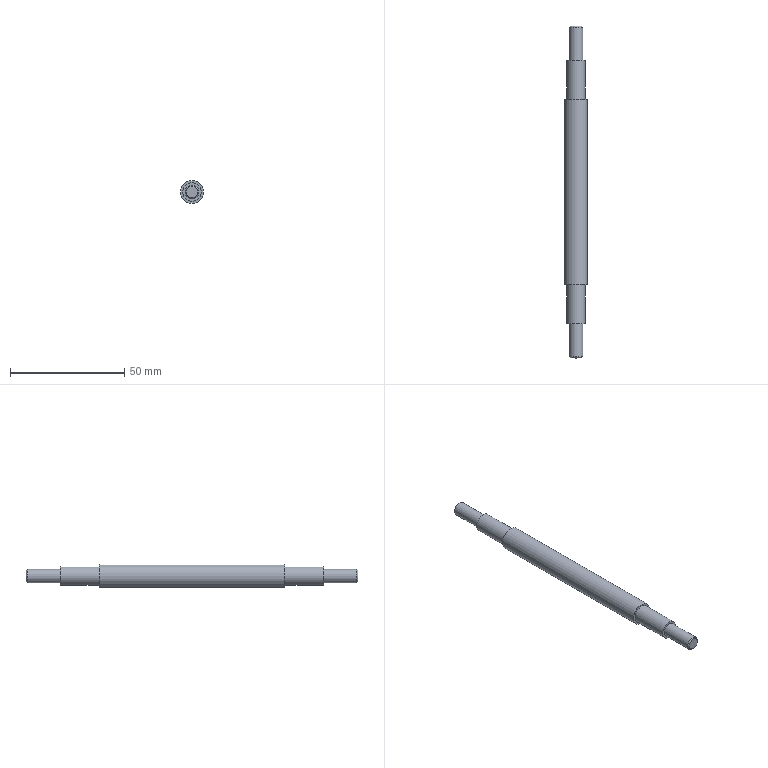Part | STEP file | 2-13.2 | 1 solid | 13 faces | box 10 x 145 x 10 mm | volume 8915 mm3 | plane 6 | cylinder 5 | cone 2 | commonest cylinder face diameters 6 x2 8 x2 10 x1
STEP:
#1=CARTESIAN_POINT('',(0.,0.,0.));
#2=DIRECTION('',(0.,0.,1.));
#3=DIRECTION('',(1.,0.,0.));
#4=AXIS2_PLACEMENT_3D('',#1,#2,#3);
#5=CARTESIAN_POINT('',(5.,40.5,0.));
#6=VERTEX_POINT('',#5);
#7=CARTESIAN_POINT('',(0.,40.5,0.));
#8=DIRECTION('',(0.,-1.,0.));
#9=DIRECTION('',(1.,0.,0.));
#10=AXIS2_PLACEMENT_3D('',#7,#8,#9);
#11=CIRCLE('',#10,5.);
#12=CARTESIAN_POINT('',(0.,40.5,0.));
#13=DIRECTION('',(0.,-1.,0.));
#14=DIRECTION('',(1.,0.,0.));
#15=AXIS2_PLACEMENT_3D('',#12,#13,#14);
#16=CYLINDRICAL_SURFACE('',#15,5.);
#17=CARTESIAN_POINT('',(0.,0.));
#18=DIRECTION('',(1.,0.));
#19=VECTOR('',#18,1.);
#20=LINE('',#17,#19);
#21=(GEOMETRIC_REPRESENTATION_CONTEXT(2)PARAMETRIC_REPRESENTATION_CONTEXT()REPRESENTATION_CONTEXT('',''));
#22=DEFINITIONAL_REPRESENTATION('',(#20),#21);
#23=PCURVE('',#16,#22);
#24=CARTESIAN_POINT('',(-1.34,40.5,0.));
#25=DIRECTION('',(0.,-1.,0.));
#26=DIRECTION('',(1.,0.,0.));
#27=AXIS2_PLACEMENT_3D('',#24,#25,#26);
#28=PLANE('',#27);
#29=CARTESIAN_POINT('',(1.34,0.));
#30=DIRECTION('',(1.,0.));
#31=AXIS2_PLACEMENT_2D('',#29,#30);
#32=CIRCLE('',#31,5.);
#33=(GEOMETRIC_REPRESENTATION_CONTEXT(2)PARAMETRIC_REPRESENTATION_CONTEXT()REPRESENTATION_CONTEXT('',''));
#34=DEFINITIONAL_REPRESENTATION('',(#32),#33);
#35=PCURVE('',#28,#34);
#36=SURFACE_CURVE('',#11,(#23,#35),.PCURVE_S1.);
#37=EDGE_CURVE('',#6,#6,#36,.T.);
#38=ORIENTED_EDGE('',*,*,#37,.T.);
#39=CARTESIAN_POINT('',(5.,-40.5,0.));
#40=VERTEX_POINT('',#39);
#41=CARTESIAN_POINT('',(5.,40.5,0.));
#42=DIRECTION('',(0.,-1.,0.));
#43=VECTOR('',#42,1.);
#44=LINE('',#41,#43);
#45=CARTESIAN_POINT('',(6.283,0.));
#46=DIRECTION('',(0.,1.));
#47=VECTOR('',#46,1.);
#48=LINE('',#45,#47);
#49=(GEOMETRIC_REPRESENTATION_CONTEXT(2)PARAMETRIC_REPRESENTATION_CONTEXT()REPRESENTATION_CONTEXT('',''));
#50=DEFINITIONAL_REPRESENTATION('',(#48),#49);
#51=PCURVE('',#16,#50);
#52=CARTESIAN_POINT('',(0.,0.));
#53=DIRECTION('',(0.,1.));
#54=VECTOR('',#53,1.);
#55=LINE('',#52,#54);
#56=(GEOMETRIC_REPRESENTATION_CONTEXT(2)PARAMETRIC_REPRESENTATION_CONTEXT()REPRESENTATION_CONTEXT('',''));
#57=DEFINITIONAL_REPRESENTATION('',(#55),#56);
#58=PCURVE('',#16,#57);
#59=SEAM_CURVE('',#44,(#51,#58),.PCURVE_S1.);
#60=EDGE_CURVE('',#6,#40,#59,.T.);
#61=ORIENTED_EDGE('',*,*,#60,.T.);
#62=CARTESIAN_POINT('',(0.,-40.5,0.));
#63=DIRECTION('',(0.,-1.,0.));
#64=DIRECTION('',(1.,0.,0.));
#65=AXIS2_PLACEMENT_3D('',#62,#63,#64);
#66=CIRCLE('',#65,5.);
#67=CARTESIAN_POINT('',(0.,81.));
#68=DIRECTION('',(1.,0.));
#69=VECTOR('',#68,1.);
#70=LINE('',#67,#69);
#71=(GEOMETRIC_REPRESENTATION_CONTEXT(2)PARAMETRIC_REPRESENTATION_CONTEXT()REPRESENTATION_CONTEXT('',''));
#72=DEFINITIONAL_REPRESENTATION('',(#70),#71);
#73=PCURVE('',#16,#72);
#74=CARTESIAN_POINT('',(-1.34,-40.5,0.));
#75=DIRECTION('',(0.,-1.,0.));
#76=DIRECTION('',(1.,0.,0.));
#77=AXIS2_PLACEMENT_3D('',#74,#75,#76);
#78=PLANE('',#77);
#79=CARTESIAN_POINT('',(1.34,0.));
#80=DIRECTION('',(1.,0.));
#81=AXIS2_PLACEMENT_2D('',#79,#80);
#82=CIRCLE('',#81,5.);
#83=(GEOMETRIC_REPRESENTATION_CONTEXT(2)PARAMETRIC_REPRESENTATION_CONTEXT()REPRESENTATION_CONTEXT('',''));
#84=DEFINITIONAL_REPRESENTATION('',(#82),#83);
#85=PCURVE('',#78,#84);
#86=SURFACE_CURVE('',#66,(#73,#85),.PCURVE_S1.);
#87=EDGE_CURVE('',#40,#40,#86,.T.);
#88=ORIENTED_EDGE('',*,*,#87,.F.);
#89=ORIENTED_EDGE('',*,*,#60,.F.);
#90=EDGE_LOOP('',(#38,#61,#88,#89));
#91=FACE_BOUND('',#90,.T.);
#92=ADVANCED_FACE('',(#91),#16,.T.);
#93=ORIENTED_EDGE('',*,*,#87,.T.);
#94=EDGE_LOOP('',(#93));
#95=FACE_BOUND('',#94,.T.);
#96=CARTESIAN_POINT('',(4.,-40.5,0.));
#97=VERTEX_POINT('',#96);
#98=CARTESIAN_POINT('',(0.,-40.5,0.));
#99=DIRECTION('',(0.,-1.,0.));
#100=DIRECTION('',(1.,0.,0.));
#101=AXIS2_PLACEMENT_3D('',#98,#99,#100);
#102=CIRCLE('',#101,4.);
#103=CARTESIAN_POINT('',(1.34,0.));
#104=DIRECTION('',(1.,0.));
#105=AXIS2_PLACEMENT_2D('',#103,#104);
#106=CIRCLE('',#105,4.);
#107=(GEOMETRIC_REPRESENTATION_CONTEXT(2)PARAMETRIC_REPRESENTATION_CONTEXT()REPRESENTATION_CONTEXT('',''));
#108=DEFINITIONAL_REPRESENTATION('',(#106),#107);
#109=PCURVE('',#78,#108);
#110=CARTESIAN_POINT('',(0.,-40.5,0.));
#111=DIRECTION('',(0.,-1.,0.));
#112=DIRECTION('',(1.,0.,0.));
#113=AXIS2_PLACEMENT_3D('',#110,#111,#112);
#114=CYLINDRICAL_SURFACE('',#113,4.);
#115=CARTESIAN_POINT('',(0.,0.));
#116=DIRECTION('',(1.,0.));
#117=VECTOR('',#116,1.);
#118=LINE('',#115,#117);
#119=(GEOMETRIC_REPRESENTATION_CONTEXT(2)PARAMETRIC_REPRESENTATION_CONTEXT()REPRESENTATION_CONTEXT('',''));
#120=DEFINITIONAL_REPRESENTATION('',(#118),#119);
#121=PCURVE('',#114,#120);
#122=SURFACE_CURVE('',#102,(#109,#121),.PCURVE_S1.);
#123=EDGE_CURVE('',#97,#97,#122,.T.);
#124=ORIENTED_EDGE('',*,*,#123,.F.);
#125=EDGE_LOOP('',(#124));
#126=FACE_BOUND('',#125,.T.);
#127=ADVANCED_FACE('',(#95,#126),#78,.T.);
#128=ORIENTED_EDGE('',*,*,#123,.T.);
#129=CARTESIAN_POINT('',(4.,-57.5,0.));
#130=VERTEX_POINT('',#129);
#131=CARTESIAN_POINT('',(4.,-40.5,0.));
#132=DIRECTION('',(0.,-1.,0.));
#133=VECTOR('',#132,1.);
#134=LINE('',#131,#133);
#135=CARTESIAN_POINT('',(6.283,0.));
#136=DIRECTION('',(0.,1.));
#137=VECTOR('',#136,1.);
#138=LINE('',#135,#137);
#139=(GEOMETRIC_REPRESENTATION_CONTEXT(2)PARAMETRIC_REPRESENTATION_CONTEXT()REPRESENTATION_CONTEXT('',''));
#140=DEFINITIONAL_REPRESENTATION('',(#138),#139);
#141=PCURVE('',#114,#140);
#142=CARTESIAN_POINT('',(0.,0.));
#143=DIRECTION('',(0.,1.));
#144=VECTOR('',#143,1.);
#145=LINE('',#142,#144);
#146=(GEOMETRIC_REPRESENTATION_CONTEXT(2)PARAMETRIC_REPRESENTATION_CONTEXT()REPRESENTATION_CONTEXT('',''));
#147=DEFINITIONAL_REPRESENTATION('',(#145),#146);
#148=PCURVE('',#114,#147);
#149=SEAM_CURVE('',#134,(#141,#148),.PCURVE_S1.);
#150=EDGE_CURVE('',#97,#130,#149,.T.);
#151=ORIENTED_EDGE('',*,*,#150,.T.);
#152=CARTESIAN_POINT('',(0.,-57.5,0.));
#153=DIRECTION('',(0.,-1.,0.));
#154=DIRECTION('',(1.,0.,0.));
#155=AXIS2_PLACEMENT_3D('',#152,#153,#154);
#156=CIRCLE('',#155,4.);
#157=CARTESIAN_POINT('',(0.,17.));
#158=DIRECTION('',(1.,0.));
#159=VECTOR('',#158,1.);
#160=LINE('',#157,#159);
#161=(GEOMETRIC_REPRESENTATION_CONTEXT(2)PARAMETRIC_REPRESENTATION_CONTEXT()REPRESENTATION_CONTEXT('',''));
#162=DEFINITIONAL_REPRESENTATION('',(#160),#161);
#163=PCURVE('',#114,#162);
#164=CARTESIAN_POINT('',(-1.072,-57.5,0.));
#165=DIRECTION('',(0.,-1.,0.));
#166=DIRECTION('',(1.,0.,0.));
#167=AXIS2_PLACEMENT_3D('',#164,#165,#166);
#168=PLANE('',#167);
#169=CARTESIAN_POINT('',(1.072,0.));
#170=DIRECTION('',(1.,0.));
#171=AXIS2_PLACEMENT_2D('',#169,#170);
#172=CIRCLE('',#171,4.);
#173=(GEOMETRIC_REPRESENTATION_CONTEXT(2)PARAMETRIC_REPRESENTATION_CONTEXT()REPRESENTATION_CONTEXT('',''));
#174=DEFINITIONAL_REPRESENTATION('',(#172),#173);
#175=PCURVE('',#168,#174);
#176=SURFACE_CURVE('',#156,(#163,#175),.PCURVE_S1.);
#177=EDGE_CURVE('',#130,#130,#176,.T.);
#178=ORIENTED_EDGE('',*,*,#177,.F.);
#179=ORIENTED_EDGE('',*,*,#150,.F.);
#180=EDGE_LOOP('',(#128,#151,#178,#179));
#181=FACE_BOUND('',#180,.T.);
#182=ADVANCED_FACE('',(#181),#114,.T.);
#183=ORIENTED_EDGE('',*,*,#177,.T.);
#184=EDGE_LOOP('',(#183));
#185=FACE_BOUND('',#184,.T.);
#186=CARTESIAN_POINT('',(3.,-57.5,0.));
#187=VERTEX_POINT('',#186);
#188=CARTESIAN_POINT('',(0.,-57.5,0.));
#189=DIRECTION('',(0.,-1.,0.));
#190=DIRECTION('',(1.,0.,0.));
#191=AXIS2_PLACEMENT_3D('',#188,#189,#190);
#192=CIRCLE('',#191,3.);
#193=CARTESIAN_POINT('',(1.072,0.));
#194=DIRECTION('',(1.,0.));
#195=AXIS2_PLACEMENT_2D('',#193,#194);
#196=CIRCLE('',#195,3.);
#197=(GEOMETRIC_REPRESENTATION_CONTEXT(2)PARAMETRIC_REPRESENTATION_CONTEXT()REPRESENTATION_CONTEXT('',''));
#198=DEFINITIONAL_REPRESENTATION('',(#196),#197);
#199=PCURVE('',#168,#198);
#200=CARTESIAN_POINT('',(0.,-57.5,0.));
#201=DIRECTION('',(0.,-1.,0.));
#202=DIRECTION('',(1.,0.,0.));
#203=AXIS2_PLACEMENT_3D('',#200,#201,#202);
#204=CYLINDRICAL_SURFACE('',#203,3.);
#205=CARTESIAN_POINT('',(0.,0.));
#206=DIRECTION('',(1.,0.));
#207=VECTOR('',#206,1.);
#208=LINE('',#205,#207);
#209=(GEOMETRIC_REPRESENTATION_CONTEXT(2)PARAMETRIC_REPRESENTATION_CONTEXT()REPRESENTATION_CONTEXT('',''));
#210=DEFINITIONAL_REPRESENTATION('',(#208),#209);
#211=PCURVE('',#204,#210);
#212=SURFACE_CURVE('',#192,(#199,#211),.PCURVE_S1.);
#213=EDGE_CURVE('',#187,#187,#212,.T.);
#214=ORIENTED_EDGE('',*,*,#213,.F.);
#215=EDGE_LOOP('',(#214));
#216=FACE_BOUND('',#215,.T.);
#217=ADVANCED_FACE('',(#185,#216),#168,.T.);
#218=ORIENTED_EDGE('',*,*,#37,.T.);
#219=EDGE_LOOP('',(#218));
#220=FACE_BOUND('',#219,.F.);
#221=CARTESIAN_POINT('',(4.,40.5,0.));
#222=VERTEX_POINT('',#221);
#223=CARTESIAN_POINT('',(0.,40.5,0.));
#224=DIRECTION('',(0.,-1.,0.));
#225=DIRECTION('',(1.,0.,0.));
#226=AXIS2_PLACEMENT_3D('',#223,#224,#225);
#227=CIRCLE('',#226,4.);
#228=CARTESIAN_POINT('',(1.34,0.));
#229=DIRECTION('',(1.,0.));
#230=AXIS2_PLACEMENT_2D('',#228,#229);
#231=CIRCLE('',#230,4.);
#232=(GEOMETRIC_REPRESENTATION_CONTEXT(2)PARAMETRIC_REPRESENTATION_CONTEXT()REPRESENTATION_CONTEXT('',''));
#233=DEFINITIONAL_REPRESENTATION('',(#231),#232);
#234=PCURVE('',#28,#233);
#235=CARTESIAN_POINT('',(0.,40.5,0.));
#236=DIRECTION('',(0.,1.,0.));
#237=DIRECTION('',(1.,0.,0.));
#238=AXIS2_PLACEMENT_3D('',#235,#236,#237);
#239=CYLINDRICAL_SURFACE('',#238,4.);
#240=CARTESIAN_POINT('',(6.283,0.));
#241=DIRECTION('',(-1.,0.));
#242=VECTOR('',#241,1.);
#243=LINE('',#240,#242);
#244=(GEOMETRIC_REPRESENTATION_CONTEXT(2)PARAMETRIC_REPRESENTATION_CONTEXT()REPRESENTATION_CONTEXT('',''));
#245=DEFINITIONAL_REPRESENTATION('',(#243),#244);
#246=PCURVE('',#239,#245);
#247=SURFACE_CURVE('',#227,(#234,#246),.PCURVE_S1.);
#248=EDGE_CURVE('',#222,#222,#247,.T.);
#249=ORIENTED_EDGE('',*,*,#248,.F.);
#250=EDGE_LOOP('',(#249));
#251=FACE_BOUND('',#250,.F.);
#252=ADVANCED_FACE('',(#220,#251),#28,.F.);
#253=CARTESIAN_POINT('',(4.,57.5,0.));
#254=VERTEX_POINT('',#253);
#255=CARTESIAN_POINT('',(4.,40.5,0.));
#256=DIRECTION('',(0.,1.,0.));
#257=VECTOR('',#256,1.);
#258=LINE('',#255,#257);
#259=CARTESIAN_POINT('',(6.283,0.));
#260=DIRECTION('',(0.,1.));
#261=VECTOR('',#260,1.);
#262=LINE('',#259,#261);
#263=(GEOMETRIC_REPRESENTATION_CONTEXT(2)PARAMETRIC_REPRESENTATION_CONTEXT()REPRESENTATION_CONTEXT('',''));
#264=DEFINITIONAL_REPRESENTATION('',(#262),#263);
#265=PCURVE('',#239,#264);
#266=CARTESIAN_POINT('',(0.,0.));
#267=DIRECTION('',(0.,1.));
#268=VECTOR('',#267,1.);
#269=LINE('',#266,#268);
#270=(GEOMETRIC_REPRESENTATION_CONTEXT(2)PARAMETRIC_REPRESENTATION_CONTEXT()REPRESENTATION_CONTEXT('',''));
#271=DEFINITIONAL_REPRESENTATION('',(#269),#270);
#272=PCURVE('',#239,#271);
#273=SEAM_CURVE('',#258,(#265,#272),.PCURVE_S1.);
#274=EDGE_CURVE('',#222,#254,#273,.T.);
#275=ORIENTED_EDGE('',*,*,#274,.T.);
#276=CARTESIAN_POINT('',(0.,57.5,0.));
#277=DIRECTION('',(0.,-1.,0.));
#278=DIRECTION('',(1.,0.,0.));
#279=AXIS2_PLACEMENT_3D('',#276,#277,#278);
#280=CIRCLE('',#279,4.);
#281=CARTESIAN_POINT('',(6.283,17.));
#282=DIRECTION('',(-1.,0.));
#283=VECTOR('',#282,1.);
#284=LINE('',#281,#283);
#285=(GEOMETRIC_REPRESENTATION_CONTEXT(2)PARAMETRIC_REPRESENTATION_CONTEXT()REPRESENTATION_CONTEXT('',''));
#286=DEFINITIONAL_REPRESENTATION('',(#284),#285);
#287=PCURVE('',#239,#286);
#288=CARTESIAN_POINT('',(-1.072,57.5,0.));
#289=DIRECTION('',(0.,-1.,0.));
#290=DIRECTION('',(1.,0.,0.));
#291=AXIS2_PLACEMENT_3D('',#288,#289,#290);
#292=PLANE('',#291);
#293=CARTESIAN_POINT('',(1.072,0.));
#294=DIRECTION('',(1.,0.));
#295=AXIS2_PLACEMENT_2D('',#293,#294);
#296=CIRCLE('',#295,4.);
#297=(GEOMETRIC_REPRESENTATION_CONTEXT(2)PARAMETRIC_REPRESENTATION_CONTEXT()REPRESENTATION_CONTEXT('',''));
#298=DEFINITIONAL_REPRESENTATION('',(#296),#297);
#299=PCURVE('',#292,#298);
#300=SURFACE_CURVE('',#280,(#287,#299),.PCURVE_S1.);
#301=EDGE_CURVE('',#254,#254,#300,.T.);
#302=ORIENTED_EDGE('',*,*,#301,.T.);
#303=ORIENTED_EDGE('',*,*,#274,.F.);
#304=ORIENTED_EDGE('',*,*,#248,.F.);
#305=EDGE_LOOP('',(#275,#302,#303,#304));
#306=FACE_BOUND('',#305,.T.);
#307=ADVANCED_FACE('',(#306),#239,.T.);
#308=ORIENTED_EDGE('',*,*,#301,.T.);
#309=EDGE_LOOP('',(#308));
#310=FACE_BOUND('',#309,.F.);
#311=CARTESIAN_POINT('',(3.,57.5,0.));
#312=VERTEX_POINT('',#311);
#313=CARTESIAN_POINT('',(0.,57.5,0.));
#314=DIRECTION('',(0.,-1.,0.));
#315=DIRECTION('',(1.,0.,0.));
#316=AXIS2_PLACEMENT_3D('',#313,#314,#315);
#317=CIRCLE('',#316,3.);
#318=CARTESIAN_POINT('',(1.072,0.));
#319=DIRECTION('',(1.,0.));
#320=AXIS2_PLACEMENT_2D('',#318,#319);
#321=CIRCLE('',#320,3.);
#322=(GEOMETRIC_REPRESENTATION_CONTEXT(2)PARAMETRIC_REPRESENTATION_CONTEXT()REPRESENTATION_CONTEXT('',''));
#323=DEFINITIONAL_REPRESENTATION('',(#321),#322);
#324=PCURVE('',#292,#323);
#325=CARTESIAN_POINT('',(0.,57.5,0.));
#326=DIRECTION('',(0.,1.,0.));
#327=DIRECTION('',(1.,0.,0.));
#328=AXIS2_PLACEMENT_3D('',#325,#326,#327);
#329=CYLINDRICAL_SURFACE('',#328,3.);
#330=CARTESIAN_POINT('',(6.283,0.));
#331=DIRECTION('',(-1.,0.));
#332=VECTOR('',#331,1.);
#333=LINE('',#330,#332);
#334=(GEOMETRIC_REPRESENTATION_CONTEXT(2)PARAMETRIC_REPRESENTATION_CONTEXT()REPRESENTATION_CONTEXT('',''));
#335=DEFINITIONAL_REPRESENTATION('',(#333),#334);
#336=PCURVE('',#329,#335);
#337=SURFACE_CURVE('',#317,(#324,#336),.PCURVE_S1.);
#338=EDGE_CURVE('',#312,#312,#337,.T.);
#339=ORIENTED_EDGE('',*,*,#338,.F.);
#340=EDGE_LOOP('',(#339));
#341=FACE_BOUND('',#340,.F.);
#342=ADVANCED_FACE('',(#310,#341),#292,.F.);
#343=ORIENTED_EDGE('',*,*,#213,.T.);
#344=CARTESIAN_POINT('',(3.,-72.,0.));
#345=VERTEX_POINT('',#344);
#346=CARTESIAN_POINT('',(3.,-57.5,0.));
#347=DIRECTION('',(0.,-1.,0.));
#348=VECTOR('',#347,1.);
#349=LINE('',#346,#348);
#350=CARTESIAN_POINT('',(6.283,0.));
#351=DIRECTION('',(0.,1.));
#352=VECTOR('',#351,1.);
#353=LINE('',#350,#352);
#354=(GEOMETRIC_REPRESENTATION_CONTEXT(2)PARAMETRIC_REPRESENTATION_CONTEXT()REPRESENTATION_CONTEXT('',''));
#355=DEFINITIONAL_REPRESENTATION('',(#353),#354);
#356=PCURVE('',#204,#355);
#357=CARTESIAN_POINT('',(0.,0.));
#358=DIRECTION('',(0.,1.));
#359=VECTOR('',#358,1.);
#360=LINE('',#357,#359);
#361=(GEOMETRIC_REPRESENTATION_CONTEXT(2)PARAMETRIC_REPRESENTATION_CONTEXT()REPRESENTATION_CONTEXT('',''));
#362=DEFINITIONAL_REPRESENTATION('',(#360),#361);
#363=PCURVE('',#204,#362);
#364=SEAM_CURVE('',#349,(#356,#363),.PCURVE_S1.);
#365=EDGE_CURVE('',#187,#345,#364,.T.);
#366=ORIENTED_EDGE('',*,*,#365,.T.);
#367=CARTESIAN_POINT('',(0.,-72.,0.));
#368=DIRECTION('',(0.,1.,0.));
#369=DIRECTION('',(1.,0.,0.));
#370=AXIS2_PLACEMENT_3D('',#367,#368,#369);
#371=CIRCLE('',#370,3.);
#372=CARTESIAN_POINT('',(6.283,14.5));
#373=DIRECTION('',(-1.,0.));
#374=VECTOR('',#373,1.);
#375=LINE('',#372,#374);
#376=(GEOMETRIC_REPRESENTATION_CONTEXT(2)PARAMETRIC_REPRESENTATION_CONTEXT()REPRESENTATION_CONTEXT('',''));
#377=DEFINITIONAL_REPRESENTATION('',(#375),#376);
#378=PCURVE('',#204,#377);
#379=CARTESIAN_POINT('',(0.,-72.5,0.));
#380=DIRECTION('',(0.,1.,0.));
#381=DIRECTION('',(1.,0.,0.));
#382=AXIS2_PLACEMENT_3D('',#379,#380,#381);
#383=CONICAL_SURFACE('',#382,2.5,0.7854);
#384=CARTESIAN_POINT('',(0.,0.5));
#385=DIRECTION('',(1.,0.));
#386=VECTOR('',#385,1.);
#387=LINE('',#384,#386);
#388=(GEOMETRIC_REPRESENTATION_CONTEXT(2)PARAMETRIC_REPRESENTATION_CONTEXT()REPRESENTATION_CONTEXT('',''));
#389=DEFINITIONAL_REPRESENTATION('',(#387),#388);
#390=PCURVE('',#383,#389);
#391=SURFACE_CURVE('',#371,(#378,#390),.PCURVE_S1.);
#392=EDGE_CURVE('',#345,#345,#391,.T.);
#393=ORIENTED_EDGE('',*,*,#392,.T.);
#394=ORIENTED_EDGE('',*,*,#365,.F.);
#395=EDGE_LOOP('',(#343,#366,#393,#394));
#396=FACE_BOUND('',#395,.T.);
#397=ADVANCED_FACE('',(#396),#204,.T.);
#398=CARTESIAN_POINT('',(2.5,-72.5,0.));
#399=VERTEX_POINT('',#398);
#400=CARTESIAN_POINT('',(0.,-72.5,0.));
#401=DIRECTION('',(0.,1.,0.));
#402=DIRECTION('',(1.,0.,0.));
#403=AXIS2_PLACEMENT_3D('',#400,#401,#402);
#404=CIRCLE('',#403,2.5);
#405=CARTESIAN_POINT('',(-0.8038,-72.5,0.));
#406=DIRECTION('',(0.,-1.,0.));
#407=DIRECTION('',(1.,0.,0.));
#408=AXIS2_PLACEMENT_3D('',#405,#406,#407);
#409=PLANE('',#408);
#410=CARTESIAN_POINT('',(3.304,0.));
#411=CARTESIAN_POINT('',(3.304,-4.33));
#412=CARTESIAN_POINT('',(-0.4462,-2.165));
#413=CARTESIAN_POINT('',(-4.196,0.));
#414=CARTESIAN_POINT('',(-0.4462,2.165));
#415=CARTESIAN_POINT('',(3.304,4.33));
#416=CARTESIAN_POINT('',(3.304,0.));
#417=(BOUNDED_CURVE()B_SPLINE_CURVE(2,(#410,#411,#412,#413,#414,#415,#416),.UNSPECIFIED.,.T.,.F.)B_SPLINE_CURVE_WITH_KNOTS((1,2,2,2,2,1),(-2.094,0.,2.094,4.189,6.283,8.378),.UNSPECIFIED.)CURVE()GEOMETRIC_REPRESENTATION_ITEM()RATIONAL_B_SPLINE_CURVE((1.,0.5,1.,0.5,1.,0.5,1.))REPRESENTATION_ITEM(''));
#418=(GEOMETRIC_REPRESENTATION_CONTEXT(2)PARAMETRIC_REPRESENTATION_CONTEXT()REPRESENTATION_CONTEXT('',''));
#419=DEFINITIONAL_REPRESENTATION('',(#417),#418);
#420=PCURVE('',#409,#419);
#421=CARTESIAN_POINT('',(0.,0.));
#422=DIRECTION('',(1.,0.));
#423=VECTOR('',#422,1.);
#424=LINE('',#421,#423);
#425=(GEOMETRIC_REPRESENTATION_CONTEXT(2)PARAMETRIC_REPRESENTATION_CONTEXT()REPRESENTATION_CONTEXT('',''));
#426=DEFINITIONAL_REPRESENTATION('',(#424),#425);
#427=PCURVE('',#383,#426);
#428=SURFACE_CURVE('',#404,(#420,#427),.PCURVE_S1.);
#429=EDGE_CURVE('',#399,#399,#428,.T.);
#430=ORIENTED_EDGE('',*,*,#429,.F.);
#431=EDGE_LOOP('',(#430));
#432=FACE_BOUND('',#431,.T.);
#433=ADVANCED_FACE('',(#432),#409,.T.);
#434=CARTESIAN_POINT('',(3.,72.,0.));
#435=VERTEX_POINT('',#434);
#436=CARTESIAN_POINT('',(3.,57.5,0.));
#437=DIRECTION('',(0.,1.,0.));
#438=VECTOR('',#437,1.);
#439=LINE('',#436,#438);
#440=CARTESIAN_POINT('',(6.283,0.));
#441=DIRECTION('',(0.,1.));
#442=VECTOR('',#441,1.);
#443=LINE('',#440,#442);
#444=(GEOMETRIC_REPRESENTATION_CONTEXT(2)PARAMETRIC_REPRESENTATION_CONTEXT()REPRESENTATION_CONTEXT('',''));
#445=DEFINITIONAL_REPRESENTATION('',(#443),#444);
#446=PCURVE('',#329,#445);
#447=CARTESIAN_POINT('',(0.,0.));
#448=DIRECTION('',(0.,1.));
#449=VECTOR('',#448,1.);
#450=LINE('',#447,#449);
#451=(GEOMETRIC_REPRESENTATION_CONTEXT(2)PARAMETRIC_REPRESENTATION_CONTEXT()REPRESENTATION_CONTEXT('',''));
#452=DEFINITIONAL_REPRESENTATION('',(#450),#451);
#453=PCURVE('',#329,#452);
#454=SEAM_CURVE('',#439,(#446,#453),.PCURVE_S1.);
#455=EDGE_CURVE('',#312,#435,#454,.T.);
#456=ORIENTED_EDGE('',*,*,#455,.T.);
#457=CARTESIAN_POINT('',(0.,72.,0.));
#458=DIRECTION('',(0.,-1.,0.));
#459=DIRECTION('',(1.,0.,0.));
#460=AXIS2_PLACEMENT_3D('',#457,#458,#459);
#461=CIRCLE('',#460,3.);
#462=CARTESIAN_POINT('',(6.283,14.5));
#463=DIRECTION('',(-1.,0.));
#464=VECTOR('',#463,1.);
#465=LINE('',#462,#464);
#466=(GEOMETRIC_REPRESENTATION_CONTEXT(2)PARAMETRIC_REPRESENTATION_CONTEXT()REPRESENTATION_CONTEXT('',''));
#467=DEFINITIONAL_REPRESENTATION('',(#465),#466);
#468=PCURVE('',#329,#467);
#469=CARTESIAN_POINT('',(0.,72.5,0.));
#470=DIRECTION('',(0.,-1.,0.));
#471=DIRECTION('',(1.,0.,0.));
#472=AXIS2_PLACEMENT_3D('',#469,#470,#471);
#473=CONICAL_SURFACE('',#472,2.5,0.7854);
#474=CARTESIAN_POINT('',(0.,0.5));
#475=DIRECTION('',(1.,0.));
#476=VECTOR('',#475,1.);
#477=LINE('',#474,#476);
#478=(GEOMETRIC_REPRESENTATION_CONTEXT(2)PARAMETRIC_REPRESENTATION_CONTEXT()REPRESENTATION_CONTEXT('',''));
#479=DEFINITIONAL_REPRESENTATION('',(#477),#478);
#480=PCURVE('',#473,#479);
#481=SURFACE_CURVE('',#461,(#468,#480),.PCURVE_S1.);
#482=EDGE_CURVE('',#435,#435,#481,.T.);
#483=ORIENTED_EDGE('',*,*,#482,.T.);
#484=ORIENTED_EDGE('',*,*,#455,.F.);
#485=ORIENTED_EDGE('',*,*,#338,.F.);
#486=EDGE_LOOP('',(#456,#483,#484,#485));
#487=FACE_BOUND('',#486,.T.);
#488=ADVANCED_FACE('',(#487),#329,.T.);
#489=CARTESIAN_POINT('',(2.5,72.5,0.));
#490=VERTEX_POINT('',#489);
#491=CARTESIAN_POINT('',(0.,72.5,0.));
#492=DIRECTION('',(0.,-1.,0.));
#493=DIRECTION('',(1.,0.,0.));
#494=AXIS2_PLACEMENT_3D('',#491,#492,#493);
#495=CIRCLE('',#494,2.5);
#496=CARTESIAN_POINT('',(-0.8038,72.5,0.));
#497=DIRECTION('',(0.,-1.,0.));
#498=DIRECTION('',(1.,0.,0.));
#499=AXIS2_PLACEMENT_3D('',#496,#497,#498);
#500=PLANE('',#499);
#501=CARTESIAN_POINT('',(0.8038,0.));
#502=DIRECTION('',(1.,0.));
#503=AXIS2_PLACEMENT_2D('',#501,#502);
#504=CIRCLE('',#503,2.5);
#505=(GEOMETRIC_REPRESENTATION_CONTEXT(2)PARAMETRIC_REPRESENTATION_CONTEXT()REPRESENTATION_CONTEXT('',''));
#506=DEFINITIONAL_REPRESENTATION('',(#504),#505);
#507=PCURVE('',#500,#506);
#508=CARTESIAN_POINT('',(0.,0.));
#509=DIRECTION('',(1.,0.));
#510=VECTOR('',#509,1.);
#511=LINE('',#508,#510);
#512=(GEOMETRIC_REPRESENTATION_CONTEXT(2)PARAMETRIC_REPRESENTATION_CONTEXT()REPRESENTATION_CONTEXT('',''));
#513=DEFINITIONAL_REPRESENTATION('',(#511),#512);
#514=PCURVE('',#473,#513);
#515=SURFACE_CURVE('',#495,(#507,#514),.PCURVE_S1.);
#516=EDGE_CURVE('',#490,#490,#515,.T.);
#517=ORIENTED_EDGE('',*,*,#516,.T.);
#518=EDGE_LOOP('',(#517));
#519=FACE_BOUND('',#518,.F.);
#520=ADVANCED_FACE('',(#519),#500,.F.);
#521=CARTESIAN_POINT('',(2.5,72.5,0.));
#522=DIRECTION('',(0.7071,-0.7071,0.));
#523=VECTOR('',#522,1.);
#524=LINE('',#521,#523);
#525=CARTESIAN_POINT('',(6.283,0.));
#526=CARTESIAN_POINT('',(6.283,0.007576));
#527=CARTESIAN_POINT('',(6.283,0.02273));
#528=CARTESIAN_POINT('',(6.283,0.04545));
#529=CARTESIAN_POINT('',(6.283,0.06818));
#530=CARTESIAN_POINT('',(6.283,0.09091));
#531=CARTESIAN_POINT('',(6.283,0.1136));
#532=CARTESIAN_POINT('',(6.283,0.1364));
#533=CARTESIAN_POINT('',(6.283,0.1591));
#534=CARTESIAN_POINT('',(6.283,0.1818));
#535=CARTESIAN_POINT('',(6.283,0.2045));
#536=CARTESIAN_POINT('',(6.283,0.2273));
#537=CARTESIAN_POINT('',(6.283,0.25));
#538=CARTESIAN_POINT('',(6.283,0.2727));
#539=CARTESIAN_POINT('',(6.283,0.2955));
#540=CARTESIAN_POINT('',(6.283,0.3182));
#541=CARTESIAN_POINT('',(6.283,0.3409));
#542=CARTESIAN_POINT('',(6.283,0.3636));
#543=CARTESIAN_POINT('',(6.283,0.3864));
#544=CARTESIAN_POINT('',(6.283,0.4091));
#545=CARTESIAN_POINT('',(6.283,0.4318));
#546=CARTESIAN_POINT('',(6.283,0.4545));
#547=CARTESIAN_POINT('',(6.283,0.4773));
#548=CARTESIAN_POINT('',(6.283,0.4924));
#549=CARTESIAN_POINT('',(6.283,0.5));
#550=B_SPLINE_CURVE_WITH_KNOTS('',3,(#525,#526,#527,#528,#529,#530,#531,#532,#533,#534,#535,#536,#537,#538,#539,#540,#541,#542,#543,#544,#545,#546,#547,#548,#549),.UNSPECIFIED.,.F.,.F.,(4,1,1,1,1,1,1,1,1,1,1,1,1,1,1,1,1,1,1,1,1,1,4),(0.,0.03214,0.06428,0.09642,0.1286,0.1607,0.1928,0.225,0.2571,0.2893,0.3214,0.3536,0.3857,0.4178,0.45,0.4821,0.5143,0.5464,0.5785,0.6107,0.6428,0.675,0.7071),.QUASI_UNIFORM_KNOTS.);
#551=(GEOMETRIC_REPRESENTATION_CONTEXT(2)PARAMETRIC_REPRESENTATION_CONTEXT()REPRESENTATION_CONTEXT('',''));
#552=DEFINITIONAL_REPRESENTATION('',(#550),#551);
#553=PCURVE('',#473,#552);
#554=CARTESIAN_POINT('',(0.,0.));
#555=CARTESIAN_POINT('',(0.,0.007576));
#556=CARTESIAN_POINT('',(0.,0.02273));
#557=CARTESIAN_POINT('',(0.,0.04545));
#558=CARTESIAN_POINT('',(0.,0.06818));
#559=CARTESIAN_POINT('',(0.,0.09091));
#560=CARTESIAN_POINT('',(0.,0.1136));
#561=CARTESIAN_POINT('',(0.,0.1364));
#562=CARTESIAN_POINT('',(0.,0.1591));
#563=CARTESIAN_POINT('',(0.,0.1818));
#564=CARTESIAN_POINT('',(0.,0.2045));
#565=CARTESIAN_POINT('',(0.,0.2273));
#566=CARTESIAN_POINT('',(0.,0.25));
#567=CARTESIAN_POINT('',(0.,0.2727));
#568=CARTESIAN_POINT('',(0.,0.2955));
#569=CARTESIAN_POINT('',(0.,0.3182));
#570=CARTESIAN_POINT('',(0.,0.3409));
#571=CARTESIAN_POINT('',(0.,0.3636));
#572=CARTESIAN_POINT('',(0.,0.3864));
#573=CARTESIAN_POINT('',(0.,0.4091));
#574=CARTESIAN_POINT('',(0.,0.4318));
#575=CARTESIAN_POINT('',(0.,0.4545));
#576=CARTESIAN_POINT('',(0.,0.4773));
#577=CARTESIAN_POINT('',(0.,0.4924));
#578=CARTESIAN_POINT('',(0.,0.5));
#579=B_SPLINE_CURVE_WITH_KNOTS('',3,(#554,#555,#556,#557,#558,#559,#560,#561,#562,#563,#564,#565,#566,#567,#568,#569,#570,#571,#572,#573,#574,#575,#576,#577,#578),.UNSPECIFIED.,.F.,.F.,(4,1,1,1,1,1,1,1,1,1,1,1,1,1,1,1,1,1,1,1,1,1,4),(0.,0.03214,0.06428,0.09642,0.1286,0.1607,0.1928,0.225,0.2571,0.2893,0.3214,0.3536,0.3857,0.4178,0.45,0.4821,0.5143,0.5464,0.5785,0.6107,0.6428,0.675,0.7071),.QUASI_UNIFORM_KNOTS.);
#580=(GEOMETRIC_REPRESENTATION_CONTEXT(2)PARAMETRIC_REPRESENTATION_CONTEXT()REPRESENTATION_CONTEXT('',''));
#581=DEFINITIONAL_REPRESENTATION('',(#579),#580);
#582=PCURVE('',#473,#581);
#583=SEAM_CURVE('',#524,(#553,#582),.PCURVE_S1.);
#584=EDGE_CURVE('',#490,#435,#583,.T.);
#585=ORIENTED_EDGE('',*,*,#584,.T.);
#586=ORIENTED_EDGE('',*,*,#482,.F.);
#587=ORIENTED_EDGE('',*,*,#584,.F.);
#588=ORIENTED_EDGE('',*,*,#516,.T.);
#589=EDGE_LOOP('',(#585,#586,#587,#588));
#590=FACE_BOUND('',#589,.T.);
#591=ADVANCED_FACE('',(#590),#473,.T.);
#592=CARTESIAN_POINT('',(2.5,-72.5,0.));
#593=DIRECTION('',(0.7071,0.7071,0.));
#594=VECTOR('',#593,1.);
#595=LINE('',#592,#594);
#596=CARTESIAN_POINT('',(6.283,0.));
#597=CARTESIAN_POINT('',(6.283,0.007576));
#598=CARTESIAN_POINT('',(6.283,0.02273));
#599=CARTESIAN_POINT('',(6.283,0.04545));
#600=CARTESIAN_POINT('',(6.283,0.06818));
#601=CARTESIAN_POINT('',(6.283,0.09091));
#602=CARTESIAN_POINT('',(6.283,0.1136));
#603=CARTESIAN_POINT('',(6.283,0.1364));
#604=CARTESIAN_POINT('',(6.283,0.1591));
#605=CARTESIAN_POINT('',(6.283,0.1818));
#606=CARTESIAN_POINT('',(6.283,0.2045));
#607=CARTESIAN_POINT('',(6.283,0.2273));
#608=CARTESIAN_POINT('',(6.283,0.25));
#609=CARTESIAN_POINT('',(6.283,0.2727));
#610=CARTESIAN_POINT('',(6.283,0.2955));
#611=CARTESIAN_POINT('',(6.283,0.3182));
#612=CARTESIAN_POINT('',(6.283,0.3409));
#613=CARTESIAN_POINT('',(6.283,0.3636));
#614=CARTESIAN_POINT('',(6.283,0.3864));
#615=CARTESIAN_POINT('',(6.283,0.4091));
#616=CARTESIAN_POINT('',(6.283,0.4318));
#617=CARTESIAN_POINT('',(6.283,0.4545));
#618=CARTESIAN_POINT('',(6.283,0.4773));
#619=CARTESIAN_POINT('',(6.283,0.4924));
#620=CARTESIAN_POINT('',(6.283,0.5));
#621=B_SPLINE_CURVE_WITH_KNOTS('',3,(#596,#597,#598,#599,#600,#601,#602,#603,#604,#605,#606,#607,#608,#609,#610,#611,#612,#613,#614,#615,#616,#617,#618,#619,#620),.UNSPECIFIED.,.F.,.F.,(4,1,1,1,1,1,1,1,1,1,1,1,1,1,1,1,1,1,1,1,1,1,4),(0.,0.03214,0.06428,0.09642,0.1286,0.1607,0.1928,0.225,0.2571,0.2893,0.3214,0.3536,0.3857,0.4178,0.45,0.4821,0.5143,0.5464,0.5785,0.6107,0.6428,0.675,0.7071),.QUASI_UNIFORM_KNOTS.);
#622=(GEOMETRIC_REPRESENTATION_CONTEXT(2)PARAMETRIC_REPRESENTATION_CONTEXT()REPRESENTATION_CONTEXT('',''));
#623=DEFINITIONAL_REPRESENTATION('',(#621),#622);
#624=PCURVE('',#383,#623);
#625=CARTESIAN_POINT('',(0.,0.));
#626=CARTESIAN_POINT('',(0.,0.007576));
#627=CARTESIAN_POINT('',(0.,0.02273));
#628=CARTESIAN_POINT('',(0.,0.04545));
#629=CARTESIAN_POINT('',(0.,0.06818));
#630=CARTESIAN_POINT('',(0.,0.09091));
#631=CARTESIAN_POINT('',(0.,0.1136));
#632=CARTESIAN_POINT('',(0.,0.1364));
#633=CARTESIAN_POINT('',(0.,0.1591));
#634=CARTESIAN_POINT('',(0.,0.1818));
#635=CARTESIAN_POINT('',(0.,0.2045));
#636=CARTESIAN_POINT('',(0.,0.2273));
#637=CARTESIAN_POINT('',(0.,0.25));
#638=CARTESIAN_POINT('',(0.,0.2727));
#639=CARTESIAN_POINT('',(0.,0.2955));
#640=CARTESIAN_POINT('',(0.,0.3182));
#641=CARTESIAN_POINT('',(0.,0.3409));
#642=CARTESIAN_POINT('',(0.,0.3636));
#643=CARTESIAN_POINT('',(0.,0.3864));
#644=CARTESIAN_POINT('',(0.,0.4091));
#645=CARTESIAN_POINT('',(0.,0.4318));
#646=CARTESIAN_POINT('',(0.,0.4545));
#647=CARTESIAN_POINT('',(0.,0.4773));
#648=CARTESIAN_POINT('',(0.,0.4924));
#649=CARTESIAN_POINT('',(0.,0.5));
#650=B_SPLINE_CURVE_WITH_KNOTS('',3,(#625,#626,#627,#628,#629,#630,#631,#632,#633,#634,#635,#636,#637,#638,#639,#640,#641,#642,#643,#644,#645,#646,#647,#648,#649),.UNSPECIFIED.,.F.,.F.,(4,1,1,1,1,1,1,1,1,1,1,1,1,1,1,1,1,1,1,1,1,1,4),(0.,0.03214,0.06428,0.09642,0.1286,0.1607,0.1928,0.225,0.2571,0.2893,0.3214,0.3536,0.3857,0.4178,0.45,0.4821,0.5143,0.5464,0.5785,0.6107,0.6428,0.675,0.7071),.QUASI_UNIFORM_KNOTS.);
#651=(GEOMETRIC_REPRESENTATION_CONTEXT(2)PARAMETRIC_REPRESENTATION_CONTEXT()REPRESENTATION_CONTEXT('',''));
#652=DEFINITIONAL_REPRESENTATION('',(#650),#651);
#653=PCURVE('',#383,#652);
#654=SEAM_CURVE('',#595,(#624,#653),.PCURVE_S1.);
#655=EDGE_CURVE('',#399,#345,#654,.T.);
#656=ORIENTED_EDGE('',*,*,#655,.T.);
#657=ORIENTED_EDGE('',*,*,#392,.F.);
#658=ORIENTED_EDGE('',*,*,#655,.F.);
#659=ORIENTED_EDGE('',*,*,#429,.T.);
#660=EDGE_LOOP('',(#656,#657,#658,#659));
#661=FACE_BOUND('',#660,.T.);
#662=ADVANCED_FACE('',(#661),#383,.T.);
#663=CLOSED_SHELL('',(#92,#127,#182,#217,#252,#307,#342,#397,#433,#488,#520,#591,#662));
#664=MANIFOLD_SOLID_BREP('',#663);
#665=(LENGTH_UNIT()NAMED_UNIT(*)SI_UNIT(.MILLI.,.METRE.));
#666=UNCERTAINTY_MEASURE_WITH_UNIT(LENGTH_MEASURE(0.0000001),#665,'','');
#667=(NAMED_UNIT(*)PLANE_ANGLE_UNIT()SI_UNIT($,.RADIAN.));
#668=(NAMED_UNIT(*)SI_UNIT($,.STERADIAN.)SOLID_ANGLE_UNIT());
#669=(GEOMETRIC_REPRESENTATION_CONTEXT(3)GLOBAL_UNCERTAINTY_ASSIGNED_CONTEXT((#666))GLOBAL_UNIT_ASSIGNED_CONTEXT((#665,#667,#668))REPRESENTATION_CONTEXT('',''));
#670=ADVANCED_BREP_SHAPE_REPRESENTATION('',(#4,#664),#669);